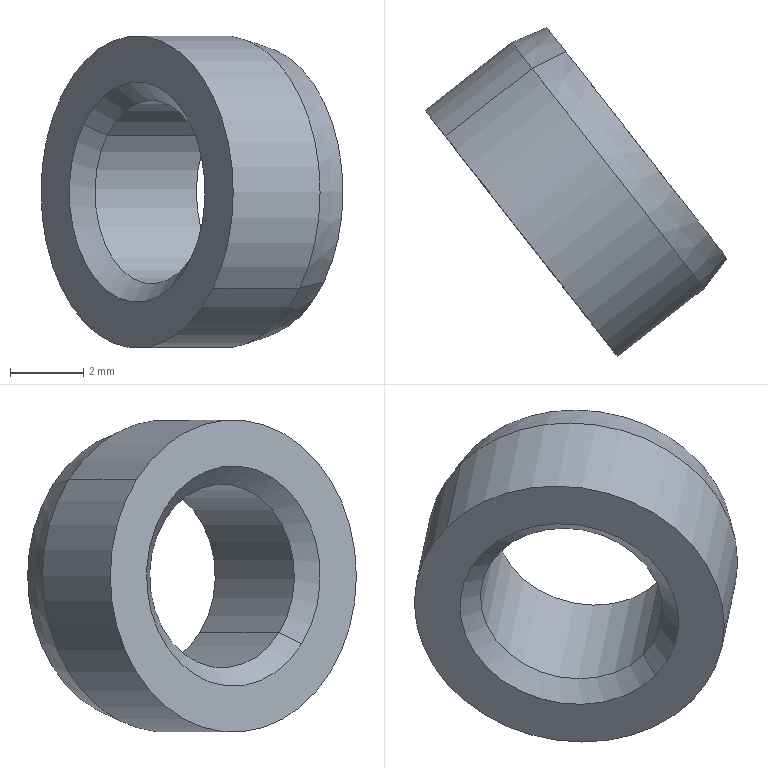Part | SolidWorks | features BaseBody 1 | 1 solid | 10 faces | box 8.22 x 8.95 x 8.5 mm | volume 142.843 mm3 | cylinder 4 | cone 4 | plane 2 | commonest cylinder face diameters 5 x2 8.5 x2
STEP:
#1=CARTESIAN_POINT('',(-16.134,83.223,-116.211));
#2=VERTEX_POINT('',#1);
#3=CARTESIAN_POINT('',(-13.708,80.118,-119.289));
#4=VERTEX_POINT('',#3);
#5=CARTESIAN_POINT('',(-14.921,81.671,-117.75));
#6=DIRECTION('',(-0.788,-0.6157,0.));
#7=DIRECTION('',(0.4851,-0.621,-0.6157));
#8=AXIS2_PLACEMENT_3D('',#5,#6,#7);
#9=CIRCLE('',#8,2.5);
#10=EDGE_CURVE('',#2,#4,#9,.T.);
#11=ORIENTED_EDGE('',*,*,#10,.F.);
#12=CARTESIAN_POINT('',(-18.892,81.068,-116.211));
#13=VERTEX_POINT('',#12);
#14=CARTESIAN_POINT('',(-19.286,80.761,-116.211));
#15=DIRECTION('',(-0.788,-0.6157,0.));
#16=VECTOR('',#15,1000.);
#17=LINE('',#14,#16);
#18=EDGE_CURVE('',#2,#13,#17,.T.);
#19=ORIENTED_EDGE('',*,*,#18,.T.);
#20=CARTESIAN_POINT('',(-16.466,77.964,-119.289));
#21=VERTEX_POINT('',#20);
#22=CARTESIAN_POINT('',(-17.679,79.516,-117.75));
#23=DIRECTION('',(-0.788,-0.6157,0.));
#24=DIRECTION('',(0.4851,-0.621,-0.6157));
#25=AXIS2_PLACEMENT_3D('',#22,#23,#24);
#26=CIRCLE('',#25,2.5);
#27=EDGE_CURVE('',#13,#21,#26,.T.);
#28=ORIENTED_EDGE('',*,*,#27,.T.);
#29=CARTESIAN_POINT('',(-16.86,77.656,-119.289));
#30=DIRECTION('',(-0.788,-0.6157,0.));
#31=VECTOR('',#30,1000.);
#32=LINE('',#29,#31);
#33=EDGE_CURVE('',#4,#21,#32,.T.);
#34=ORIENTED_EDGE('',*,*,#33,.F.);
#35=EDGE_LOOP('',(#11,#19,#28,#34));
#36=FACE_OUTER_BOUND('',#35,.T.);
#37=CARTESIAN_POINT('',(-18.073,79.208,-117.75));
#38=DIRECTION('',(-0.788,-0.6157,0.));
#39=DIRECTION('',(0.4851,-0.621,-0.6157));
#40=AXIS2_PLACEMENT_3D('',#37,#38,#39);
#41=CYLINDRICAL_SURFACE('',#40,2.5);
#42=ADVANCED_FACE('',(#36),#41,.F.);
#43=CARTESIAN_POINT('',(-13.647,78.416,-120.367));
#44=VERTEX_POINT('',#43);
#45=CARTESIAN_POINT('',(-17.771,83.694,-115.133));
#46=VERTEX_POINT('',#45);
#47=CARTESIAN_POINT('',(-15.709,81.055,-117.75));
#48=DIRECTION('',(-0.788,-0.6157,0.));
#49=DIRECTION('',(0.4851,-0.621,-0.6157));
#50=AXIS2_PLACEMENT_3D('',#47,#48,#49);
#51=CIRCLE('',#50,4.25);
#52=EDGE_CURVE('',#44,#46,#51,.T.);
#53=ORIENTED_EDGE('',*,*,#52,.T.);
#54=CARTESIAN_POINT('',(-20.135,81.847,-115.133));
#55=VERTEX_POINT('',#54);
#56=CARTESIAN_POINT('',(-20.135,81.847,-115.133));
#57=DIRECTION('',(-0.788,-0.6157,0.));
#58=VECTOR('',#57,1000.);
#59=LINE('',#56,#58);
#60=EDGE_CURVE('',#46,#55,#59,.T.);
#61=ORIENTED_EDGE('',*,*,#60,.T.);
#62=CARTESIAN_POINT('',(-16.011,76.569,-120.367));
#63=VERTEX_POINT('',#62);
#64=CARTESIAN_POINT('',(-18.073,79.208,-117.75));
#65=DIRECTION('',(-0.788,-0.6157,0.));
#66=DIRECTION('',(0.4851,-0.621,-0.6157));
#67=AXIS2_PLACEMENT_3D('',#64,#65,#66);
#68=CIRCLE('',#67,4.25);
#69=EDGE_CURVE('',#63,#55,#68,.T.);
#70=ORIENTED_EDGE('',*,*,#69,.F.);
#71=CARTESIAN_POINT('',(-16.011,76.569,-120.367));
#72=DIRECTION('',(-0.788,-0.6157,0.));
#73=VECTOR('',#72,1000.);
#74=LINE('',#71,#73);
#75=EDGE_CURVE('',#44,#63,#74,.T.);
#76=ORIENTED_EDGE('',*,*,#75,.F.);
#77=EDGE_LOOP('',(#53,#61,#70,#76));
#78=FACE_OUTER_BOUND('',#77,.T.);
#79=CARTESIAN_POINT('',(-18.073,79.208,-117.75));
#80=DIRECTION('',(-0.788,-0.6157,0.));
#81=DIRECTION('',(0.4851,-0.621,-0.6157));
#82=AXIS2_PLACEMENT_3D('',#79,#80,#81);
#83=CYLINDRICAL_SURFACE('',#82,4.25);
#84=ADVANCED_FACE('',(#78),#83,.T.);
#85=CARTESIAN_POINT('',(-12.989,79.198,-120.202));
#86=VERTEX_POINT('',#85);
#87=CARTESIAN_POINT('',(-16.853,84.144,-115.298));
#88=VERTEX_POINT('',#87);
#89=CARTESIAN_POINT('',(-14.921,81.671,-117.75));
#90=DIRECTION('',(-0.788,-0.6157,0.));
#91=DIRECTION('',(0.4851,-0.621,-0.6157));
#92=AXIS2_PLACEMENT_3D('',#89,#90,#91);
#93=CIRCLE('',#92,3.982);
#94=EDGE_CURVE('',#86,#88,#93,.T.);
#95=ORIENTED_EDGE('',*,*,#94,.T.);
#96=CARTESIAN_POINT('',(-17.771,83.694,-115.133));
#97=DIRECTION('',(-0.8867,-0.434,0.1593));
#98=VECTOR('',#97,1000.);
#99=LINE('',#96,#98);
#100=EDGE_CURVE('',#88,#46,#99,.T.);
#101=ORIENTED_EDGE('',*,*,#100,.T.);
#102=ORIENTED_EDGE('',*,*,#52,.F.);
#103=CARTESIAN_POINT('',(-13.647,78.416,-120.367));
#104=DIRECTION('',(-0.6356,-0.7554,-0.1593));
#105=VECTOR('',#104,1000.);
#106=LINE('',#103,#105);
#107=EDGE_CURVE('',#86,#44,#106,.T.);
#108=ORIENTED_EDGE('',*,*,#107,.F.);
#109=EDGE_LOOP('',(#95,#101,#102,#108));
#110=FACE_OUTER_BOUND('',#109,.T.);
#111=CARTESIAN_POINT('',(-15.709,81.055,-117.75));
#112=DIRECTION('',(-0.788,-0.6157,0.));
#113=DIRECTION('',(0.4851,-0.621,-0.6157));
#114=AXIS2_PLACEMENT_3D('',#111,#112,#113);
#115=CONICAL_SURFACE('',#114,4.25,0.2618);
#116=ADVANCED_FACE('',(#110),#115,.T.);
#117=ORIENTED_EDGE('',*,*,#27,.F.);
#118=CARTESIAN_POINT('',(-19.528,81.071,-115.903));
#119=VERTEX_POINT('',#118);
#120=CARTESIAN_POINT('',(-18.892,81.068,-116.211));
#121=DIRECTION('',(-0.9003,0.003747,0.4353));
#122=VECTOR('',#121,1000.);
#123=LINE('',#120,#122);
#124=EDGE_CURVE('',#13,#119,#123,.T.);
#125=ORIENTED_EDGE('',*,*,#124,.T.);
#126=CARTESIAN_POINT('',(-16.618,77.345,-119.597));
#127=VERTEX_POINT('',#126);
#128=CARTESIAN_POINT('',(-18.073,79.208,-117.75));
#129=DIRECTION('',(0.788,0.6157,0.));
#130=DIRECTION('',(0.4851,-0.621,-0.6157));
#131=AXIS2_PLACEMENT_3D('',#128,#129,#130);
#132=CIRCLE('',#131,3.);
#133=EDGE_CURVE('',#127,#119,#132,.T.);
#134=ORIENTED_EDGE('',*,*,#133,.F.);
#135=CARTESIAN_POINT('',(-16.466,77.964,-119.289));
#136=DIRECTION('',(-0.2142,-0.8744,-0.4353));
#137=VECTOR('',#136,1000.);
#138=LINE('',#135,#137);
#139=EDGE_CURVE('',#21,#127,#138,.T.);
#140=ORIENTED_EDGE('',*,*,#139,.F.);
#141=EDGE_LOOP('',(#117,#125,#134,#140));
#142=FACE_OUTER_BOUND('',#141,.T.);
#143=CARTESIAN_POINT('',(-17.679,79.516,-117.75));
#144=DIRECTION('',(-0.788,-0.6157,0.));
#145=DIRECTION('',(0.4851,-0.621,-0.6157));
#146=AXIS2_PLACEMENT_3D('',#143,#144,#145);
#147=CONICAL_SURFACE('',#146,2.5,0.7854);
#148=ADVANCED_FACE('',(#142),#147,.F.);
#149=ORIENTED_EDGE('',*,*,#124,.F.);
#150=CARTESIAN_POINT('',(-17.679,79.516,-117.75));
#151=DIRECTION('',(-0.788,-0.6157,0.));
#152=DIRECTION('',(0.4851,-0.621,-0.6157));
#153=AXIS2_PLACEMENT_3D('',#150,#151,#152);
#154=CIRCLE('',#153,2.5);
#155=EDGE_CURVE('',#21,#13,#154,.T.);
#156=ORIENTED_EDGE('',*,*,#155,.F.);
#157=ORIENTED_EDGE('',*,*,#139,.T.);
#158=CARTESIAN_POINT('',(-18.073,79.208,-117.75));
#159=DIRECTION('',(0.788,0.6157,0.));
#160=DIRECTION('',(0.4851,-0.621,-0.6157));
#161=AXIS2_PLACEMENT_3D('',#158,#159,#160);
#162=CIRCLE('',#161,3.);
#163=EDGE_CURVE('',#119,#127,#162,.T.);
#164=ORIENTED_EDGE('',*,*,#163,.F.);
#165=EDGE_LOOP('',(#149,#156,#157,#164));
#166=FACE_OUTER_BOUND('',#165,.T.);
#167=CARTESIAN_POINT('',(-17.679,79.516,-117.75));
#168=DIRECTION('',(-0.788,-0.6157,0.));
#169=DIRECTION('',(0.4851,-0.621,-0.6157));
#170=AXIS2_PLACEMENT_3D('',#167,#168,#169);
#171=CONICAL_SURFACE('',#170,2.5,0.7854);
#172=ADVANCED_FACE('',(#166),#171,.F.);
#173=ORIENTED_EDGE('',*,*,#94,.F.);
#174=CARTESIAN_POINT('',(-14.921,81.671,-117.75));
#175=DIRECTION('',(-0.788,-0.6157,0.));
#176=DIRECTION('',(0.4851,-0.621,-0.6157));
#177=AXIS2_PLACEMENT_3D('',#174,#175,#176);
#178=CIRCLE('',#177,3.982);
#179=EDGE_CURVE('',#88,#86,#178,.T.);
#180=ORIENTED_EDGE('',*,*,#179,.F.);
#181=EDGE_LOOP('',(#173,#180));
#182=FACE_OUTER_BOUND('',#181,.T.);
#183=CARTESIAN_POINT('',(-14.921,81.671,-117.75));
#184=DIRECTION('',(-0.788,-0.6157,0.));
#185=DIRECTION('',(0.4851,-0.621,-0.6157));
#186=AXIS2_PLACEMENT_3D('',#183,#184,#185);
#187=CIRCLE('',#186,2.5);
#188=EDGE_CURVE('',#4,#2,#187,.T.);
#189=ORIENTED_EDGE('',*,*,#188,.T.);
#190=ORIENTED_EDGE('',*,*,#10,.T.);
#191=EDGE_LOOP('',(#189,#190));
#192=FACE_BOUND('',#191,.T.);
#193=CARTESIAN_POINT('',(-13.412,79.739,-114.612));
#194=DIRECTION('',(0.788,0.6157,0.));
#195=DIRECTION('',(0.,0.,-1.));
#196=AXIS2_PLACEMENT_3D('',#193,#194,#195);
#197=PLANE('',#196);
#198=ADVANCED_FACE('',(#182,#192),#197,.T.);
#199=ORIENTED_EDGE('',*,*,#100,.F.);
#200=ORIENTED_EDGE('',*,*,#179,.T.);
#201=ORIENTED_EDGE('',*,*,#107,.T.);
#202=CARTESIAN_POINT('',(-15.709,81.055,-117.75));
#203=DIRECTION('',(-0.788,-0.6157,0.));
#204=DIRECTION('',(0.4851,-0.621,-0.6157));
#205=AXIS2_PLACEMENT_3D('',#202,#203,#204);
#206=CIRCLE('',#205,4.25);
#207=EDGE_CURVE('',#46,#44,#206,.T.);
#208=ORIENTED_EDGE('',*,*,#207,.F.);
#209=EDGE_LOOP('',(#199,#200,#201,#208));
#210=FACE_OUTER_BOUND('',#209,.T.);
#211=CARTESIAN_POINT('',(-15.709,81.055,-117.75));
#212=DIRECTION('',(-0.788,-0.6157,0.));
#213=DIRECTION('',(0.4851,-0.621,-0.6157));
#214=AXIS2_PLACEMENT_3D('',#211,#212,#213);
#215=CONICAL_SURFACE('',#214,4.25,0.2618);
#216=ADVANCED_FACE('',(#210),#215,.T.);
#217=ORIENTED_EDGE('',*,*,#60,.F.);
#218=ORIENTED_EDGE('',*,*,#207,.T.);
#219=ORIENTED_EDGE('',*,*,#75,.T.);
#220=CARTESIAN_POINT('',(-18.073,79.208,-117.75));
#221=DIRECTION('',(-0.788,-0.6157,0.));
#222=DIRECTION('',(0.4851,-0.621,-0.6157));
#223=AXIS2_PLACEMENT_3D('',#220,#221,#222);
#224=CIRCLE('',#223,4.25);
#225=EDGE_CURVE('',#55,#63,#224,.T.);
#226=ORIENTED_EDGE('',*,*,#225,.F.);
#227=EDGE_LOOP('',(#217,#218,#219,#226));
#228=FACE_OUTER_BOUND('',#227,.T.);
#229=CARTESIAN_POINT('',(-18.073,79.208,-117.75));
#230=DIRECTION('',(-0.788,-0.6157,0.));
#231=DIRECTION('',(0.4851,-0.621,-0.6157));
#232=AXIS2_PLACEMENT_3D('',#229,#230,#231);
#233=CYLINDRICAL_SURFACE('',#232,4.25);
#234=ADVANCED_FACE('',(#228),#233,.T.);
#235=ORIENTED_EDGE('',*,*,#69,.T.);
#236=ORIENTED_EDGE('',*,*,#225,.T.);
#237=EDGE_LOOP('',(#235,#236));
#238=FACE_OUTER_BOUND('',#237,.T.);
#239=ORIENTED_EDGE('',*,*,#133,.T.);
#240=ORIENTED_EDGE('',*,*,#163,.T.);
#241=EDGE_LOOP('',(#239,#240));
#242=FACE_BOUND('',#241,.T.);
#243=CARTESIAN_POINT('',(-17.125,77.995,-115.78));
#244=DIRECTION('',(-0.788,-0.6157,0.));
#245=DIRECTION('',(-0.6157,0.788,0.));
#246=AXIS2_PLACEMENT_3D('',#243,#244,#245);
#247=PLANE('',#246);
#248=ADVANCED_FACE('',(#238,#242),#247,.T.);
#249=ORIENTED_EDGE('',*,*,#18,.F.);
#250=ORIENTED_EDGE('',*,*,#188,.F.);
#251=ORIENTED_EDGE('',*,*,#33,.T.);
#252=ORIENTED_EDGE('',*,*,#155,.T.);
#253=EDGE_LOOP('',(#249,#250,#251,#252));
#254=FACE_OUTER_BOUND('',#253,.T.);
#255=CARTESIAN_POINT('',(-18.073,79.208,-117.75));
#256=DIRECTION('',(-0.788,-0.6157,0.));
#257=DIRECTION('',(0.4851,-0.621,-0.6157));
#258=AXIS2_PLACEMENT_3D('',#255,#256,#257);
#259=CYLINDRICAL_SURFACE('',#258,2.5);
#260=ADVANCED_FACE('',(#254),#259,.F.);
#261=CLOSED_SHELL('',(#42,#84,#116,#148,#172,#198,#216,#234,#248,#260));
#262=MANIFOLD_SOLID_BREP('',#261);
#263=CARTESIAN_POINT('',(0.,0.,0.));
#264=DIRECTION('',(0.,0.,1.));
#265=DIRECTION('',(1.,0.,0.));
#266=AXIS2_PLACEMENT_3D('',#263,#264,#265);
#267=(LENGTH_UNIT()NAMED_UNIT(*)SI_UNIT(.MILLI.,.METRE.));
#268=UNCERTAINTY_MEASURE_WITH_UNIT(LENGTH_MEASURE(0.00001),#267,'','');
#269=(NAMED_UNIT(*)PLANE_ANGLE_UNIT()SI_UNIT($,.RADIAN.));
#270=(NAMED_UNIT(*)SI_UNIT($,.STERADIAN.)SOLID_ANGLE_UNIT());
#271=(GEOMETRIC_REPRESENTATION_CONTEXT(3)GLOBAL_UNCERTAINTY_ASSIGNED_CONTEXT((#268))GLOBAL_UNIT_ASSIGNED_CONTEXT((#267,#269,#270))REPRESENTATION_CONTEXT('',''));
#272=ADVANCED_BREP_SHAPE_REPRESENTATION('',(#262,#266),#271);